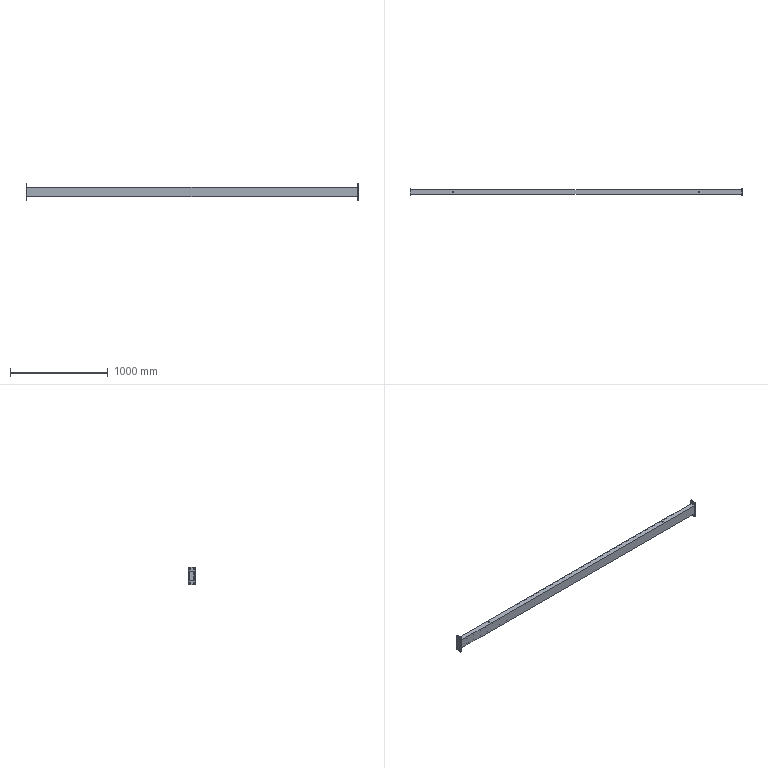Part | SolidWorks | features ICE 2, MirrorSolid 1, PLine 1, WeldMemberFeat 1, WeldmentFeature 1 | 3 solids | 56 faces | box 3391 x 70 x 180 mm | volume 4531337 mm3 | cylinder 32 | plane 24 | commonest cylinder face diameters 14 x16 20 x8 12 x4 8.4 x2 17 x2